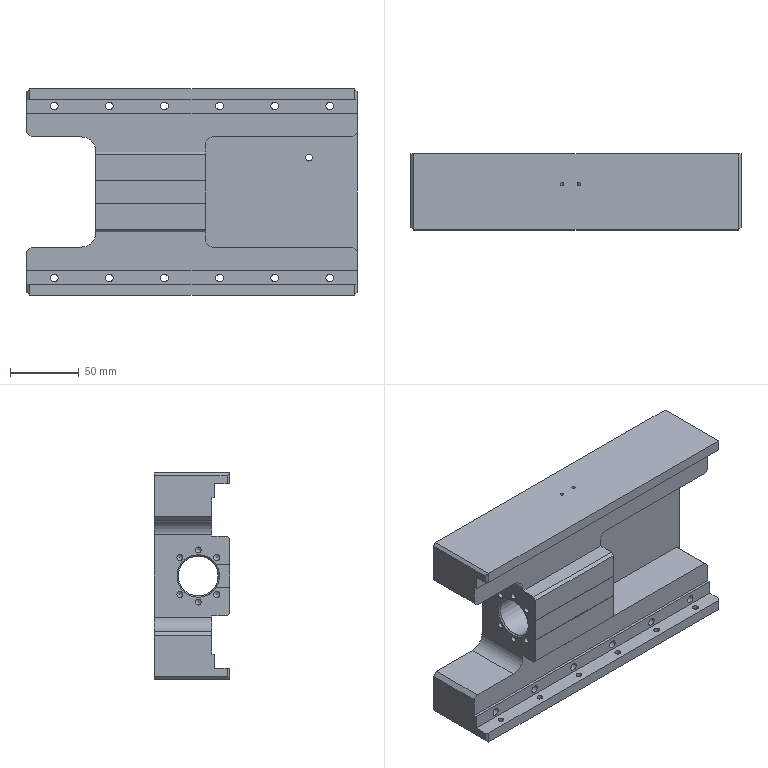Part | 2 solids | 265 faces | box 240 x 55 x 150 mm | volume 2232905 mm3 | cylinder 112 | plane 109 | cone 44 | commonest cylinder face diameters 4.2 x32 10 x28 5.5 x24 5 x12 2.5 x4 6 x4